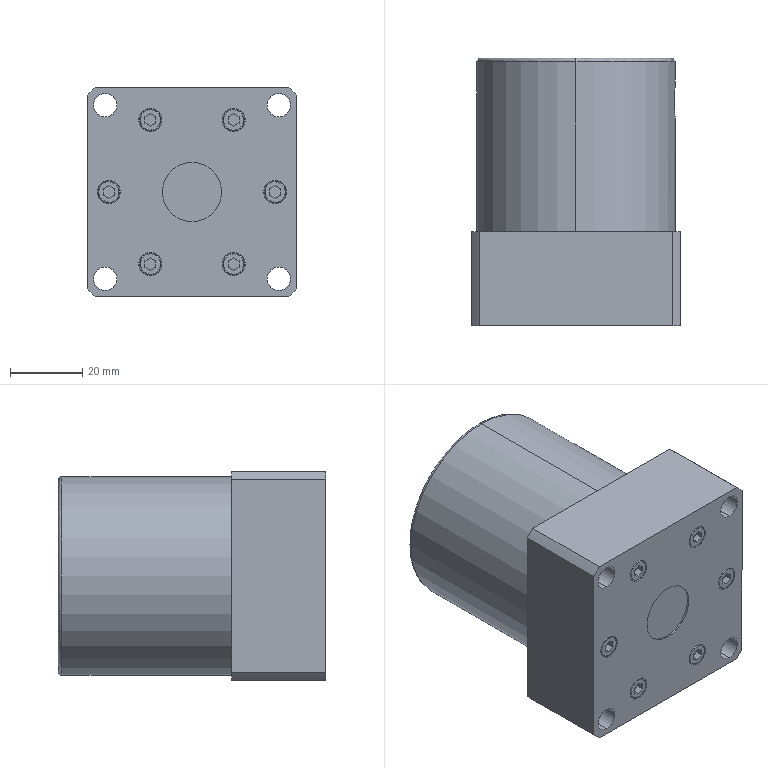Part | SolidWorks | features BaseBody 1 | 1 solid | 134 faces | box 58 x 74 x 58 mm | volume 141340 mm3 | plane 64 | cylinder 48 | spline 14 | cone 8 | commonest cylinder face diameters 6 x12 6.4 x12 6.5 x8 8.566 x4 79 x4 16 x2